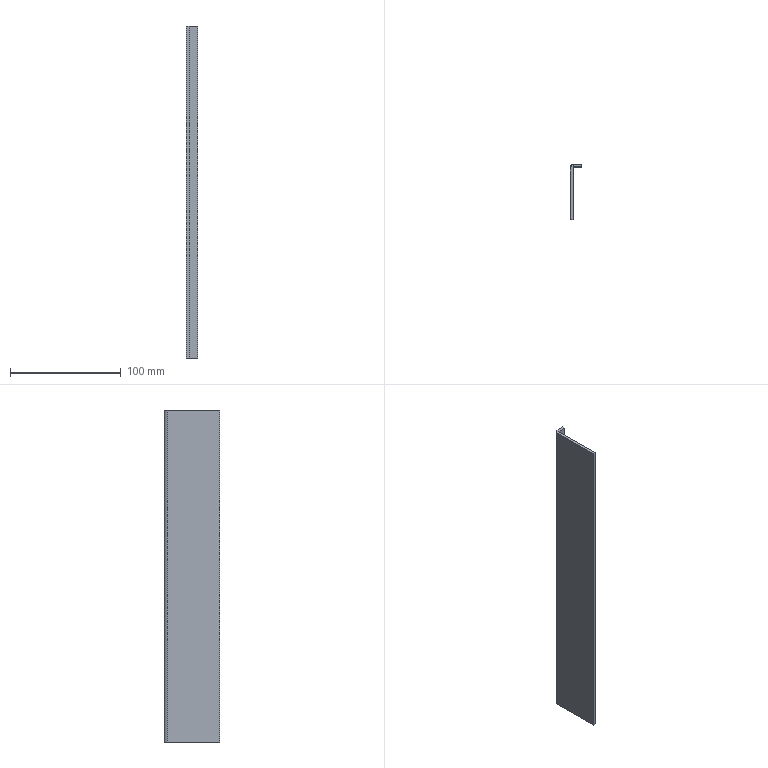Part | SolidWorks | features FlatPattern 1, SMBaseFlange 1, SheetMetal 1 | 1 solid | 14 faces | box 10 x 49.9 x 300 mm | volume 42615 mm3 | plane 12 | cylinder 2 | commonest cylinder face diameters 0.2 x1 5.2 x1
STEP:
#1=CARTESIAN_POINT('',(-7.4,0.,300.));
#2=VERTEX_POINT('',#1);
#3=CARTESIAN_POINT('',(-7.4,-2.5,300.));
#4=VERTEX_POINT('',#3);
#5=CARTESIAN_POINT('',(-7.4,0.,300.));
#6=DIRECTION('',(0.,-1.,0.));
#7=VECTOR('',#6,1000.);
#8=LINE('',#5,#7);
#9=EDGE_CURVE('',#2,#4,#8,.T.);
#10=ORIENTED_EDGE('',*,*,#9,.F.);
#11=CARTESIAN_POINT('',(-10.,-2.6,300.));
#12=VERTEX_POINT('',#11);
#13=CARTESIAN_POINT('',(-7.4,-2.6,300.));
#14=DIRECTION('',(0.,0.,1.));
#15=DIRECTION('',(-1.,0.,0.));
#16=AXIS2_PLACEMENT_3D('',#13,#14,#15);
#17=CIRCLE('',#16,2.6);
#18=EDGE_CURVE('',#2,#12,#17,.T.);
#19=ORIENTED_EDGE('',*,*,#18,.T.);
#20=CARTESIAN_POINT('',(-7.5,-2.6,300.));
#21=VERTEX_POINT('',#20);
#22=CARTESIAN_POINT('',(-7.5,-2.6,300.));
#23=DIRECTION('',(-1.,0.,0.));
#24=VECTOR('',#23,1000.);
#25=LINE('',#22,#24);
#26=EDGE_CURVE('',#21,#12,#25,.T.);
#27=ORIENTED_EDGE('',*,*,#26,.F.);
#28=CARTESIAN_POINT('',(-7.4,-2.6,300.));
#29=DIRECTION('',(0.,0.,1.));
#30=DIRECTION('',(1.,0.,0.));
#31=AXIS2_PLACEMENT_3D('',#28,#29,#30);
#32=CIRCLE('',#31,0.1);
#33=EDGE_CURVE('',#4,#21,#32,.T.);
#34=ORIENTED_EDGE('',*,*,#33,.F.);
#35=EDGE_LOOP('',(#10,#19,#27,#34));
#36=FACE_OUTER_BOUND('',#35,.T.);
#37=CARTESIAN_POINT('',(-7.4,0.,300.));
#38=DIRECTION('',(0.,0.,1.));
#39=DIRECTION('',(1.,0.,0.));
#40=AXIS2_PLACEMENT_3D('',#37,#38,#39);
#41=PLANE('',#40);
#42=ADVANCED_FACE('',(#36),#41,.T.);
#43=CARTESIAN_POINT('',(0.,0.,300.));
#44=VERTEX_POINT('',#43);
#45=CARTESIAN_POINT('',(0.,0.,300.));
#46=DIRECTION('',(-1.,0.,0.));
#47=VECTOR('',#46,1000.);
#48=LINE('',#45,#47);
#49=EDGE_CURVE('',#44,#2,#48,.T.);
#50=ORIENTED_EDGE('',*,*,#49,.T.);
#51=ORIENTED_EDGE('',*,*,#9,.T.);
#52=CARTESIAN_POINT('',(0.,-2.5,300.));
#53=VERTEX_POINT('',#52);
#54=CARTESIAN_POINT('',(0.,-2.5,300.));
#55=DIRECTION('',(-1.,0.,0.));
#56=VECTOR('',#55,1000.);
#57=LINE('',#54,#56);
#58=EDGE_CURVE('',#53,#4,#57,.T.);
#59=ORIENTED_EDGE('',*,*,#58,.F.);
#60=CARTESIAN_POINT('',(0.,0.,300.));
#61=DIRECTION('',(0.,-1.,0.));
#62=VECTOR('',#61,1000.);
#63=LINE('',#60,#62);
#64=EDGE_CURVE('',#44,#53,#63,.T.);
#65=ORIENTED_EDGE('',*,*,#64,.F.);
#66=EDGE_LOOP('',(#50,#51,#59,#65));
#67=FACE_OUTER_BOUND('',#66,.T.);
#68=CARTESIAN_POINT('',(-7.5,-2.6,300.));
#69=DIRECTION('',(0.,0.,1.));
#70=DIRECTION('',(1.,0.,0.));
#71=AXIS2_PLACEMENT_3D('',#68,#69,#70);
#72=PLANE('',#71);
#73=ADVANCED_FACE('',(#67),#72,.T.);
#74=CARTESIAN_POINT('',(-10.,-2.6,0.));
#75=VERTEX_POINT('',#74);
#76=CARTESIAN_POINT('',(-7.5,-2.6,0.));
#77=VERTEX_POINT('',#76);
#78=CARTESIAN_POINT('',(-10.,-2.6,0.));
#79=DIRECTION('',(1.,0.,0.));
#80=VECTOR('',#79,1000.);
#81=LINE('',#78,#80);
#82=EDGE_CURVE('',#75,#77,#81,.T.);
#83=ORIENTED_EDGE('',*,*,#82,.F.);
#84=CARTESIAN_POINT('',(-7.4,0.,0.));
#85=VERTEX_POINT('',#84);
#86=CARTESIAN_POINT('',(-7.4,-2.6,0.));
#87=DIRECTION('',(0.,0.,1.));
#88=DIRECTION('',(-1.,0.,0.));
#89=AXIS2_PLACEMENT_3D('',#86,#87,#88);
#90=CIRCLE('',#89,2.6);
#91=EDGE_CURVE('',#85,#75,#90,.T.);
#92=ORIENTED_EDGE('',*,*,#91,.F.);
#93=CARTESIAN_POINT('',(-7.4,-2.5,0.));
#94=VERTEX_POINT('',#93);
#95=CARTESIAN_POINT('',(-7.4,-2.5,0.));
#96=DIRECTION('',(0.,1.,0.));
#97=VECTOR('',#96,1000.);
#98=LINE('',#95,#97);
#99=EDGE_CURVE('',#94,#85,#98,.T.);
#100=ORIENTED_EDGE('',*,*,#99,.F.);
#101=CARTESIAN_POINT('',(-7.4,-2.6,0.));
#102=DIRECTION('',(0.,0.,1.));
#103=DIRECTION('',(1.,0.,0.));
#104=AXIS2_PLACEMENT_3D('',#101,#102,#103);
#105=CIRCLE('',#104,0.1);
#106=EDGE_CURVE('',#94,#77,#105,.T.);
#107=ORIENTED_EDGE('',*,*,#106,.T.);
#108=EDGE_LOOP('',(#83,#92,#100,#107));
#109=FACE_OUTER_BOUND('',#108,.T.);
#110=CARTESIAN_POINT('',(-10.,-2.6,0.));
#111=DIRECTION('',(0.,0.,-1.));
#112=DIRECTION('',(-1.,0.,0.));
#113=AXIS2_PLACEMENT_3D('',#110,#111,#112);
#114=PLANE('',#113);
#115=ADVANCED_FACE('',(#109),#114,.T.);
#116=CARTESIAN_POINT('',(-10.,-49.9,0.));
#117=VERTEX_POINT('',#116);
#118=CARTESIAN_POINT('',(-10.,0.,0.));
#119=DIRECTION('',(0.,-1.,0.));
#120=VECTOR('',#119,1000.);
#121=LINE('',#118,#120);
#122=EDGE_CURVE('',#75,#117,#121,.T.);
#123=ORIENTED_EDGE('',*,*,#122,.F.);
#124=ORIENTED_EDGE('',*,*,#82,.T.);
#125=CARTESIAN_POINT('',(-7.5,-49.9,0.));
#126=VERTEX_POINT('',#125);
#127=CARTESIAN_POINT('',(-7.5,0.,0.));
#128=DIRECTION('',(0.,-1.,0.));
#129=VECTOR('',#128,1000.);
#130=LINE('',#127,#129);
#131=EDGE_CURVE('',#77,#126,#130,.T.);
#132=ORIENTED_EDGE('',*,*,#131,.T.);
#133=CARTESIAN_POINT('',(-7.5,-49.9,0.));
#134=DIRECTION('',(-1.,0.,0.));
#135=VECTOR('',#134,1000.);
#136=LINE('',#133,#135);
#137=EDGE_CURVE('',#126,#117,#136,.T.);
#138=ORIENTED_EDGE('',*,*,#137,.T.);
#139=EDGE_LOOP('',(#123,#124,#132,#138));
#140=FACE_OUTER_BOUND('',#139,.T.);
#141=CARTESIAN_POINT('',(-7.4,-2.5,0.));
#142=DIRECTION('',(0.,0.,-1.));
#143=DIRECTION('',(-1.,0.,0.));
#144=AXIS2_PLACEMENT_3D('',#141,#142,#143);
#145=PLANE('',#144);
#146=ADVANCED_FACE('',(#140),#145,.T.);
#147=ORIENTED_EDGE('',*,*,#122,.T.);
#148=CARTESIAN_POINT('',(-10.,-49.9,300.));
#149=VERTEX_POINT('',#148);
#150=CARTESIAN_POINT('',(-10.,-49.9,300.));
#151=DIRECTION('',(0.,0.,-1.));
#152=VECTOR('',#151,1000.);
#153=LINE('',#150,#152);
#154=EDGE_CURVE('',#149,#117,#153,.T.);
#155=ORIENTED_EDGE('',*,*,#154,.F.);
#156=CARTESIAN_POINT('',(-10.,0.,300.));
#157=DIRECTION('',(0.,-1.,0.));
#158=VECTOR('',#157,1000.);
#159=LINE('',#156,#158);
#160=EDGE_CURVE('',#12,#149,#159,.T.);
#161=ORIENTED_EDGE('',*,*,#160,.F.);
#162=CARTESIAN_POINT('',(-10.,-2.6,300.));
#163=DIRECTION('',(0.,0.,-1.));
#164=VECTOR('',#163,1000.);
#165=LINE('',#162,#164);
#166=EDGE_CURVE('',#12,#75,#165,.T.);
#167=ORIENTED_EDGE('',*,*,#166,.T.);
#168=EDGE_LOOP('',(#147,#155,#161,#167));
#169=FACE_OUTER_BOUND('',#168,.T.);
#170=CARTESIAN_POINT('',(-10.,0.,300.));
#171=DIRECTION('',(1.,0.,0.));
#172=DIRECTION('',(0.,1.,0.));
#173=AXIS2_PLACEMENT_3D('',#170,#171,#172);
#174=PLANE('',#173);
#175=ADVANCED_FACE('',(#169),#174,.F.);
#176=ORIENTED_EDGE('',*,*,#137,.F.);
#177=CARTESIAN_POINT('',(-7.5,-49.9,300.));
#178=VERTEX_POINT('',#177);
#179=CARTESIAN_POINT('',(-7.5,-49.9,300.));
#180=DIRECTION('',(0.,0.,-1.));
#181=VECTOR('',#180,1000.);
#182=LINE('',#179,#181);
#183=EDGE_CURVE('',#178,#126,#182,.T.);
#184=ORIENTED_EDGE('',*,*,#183,.F.);
#185=CARTESIAN_POINT('',(-7.5,-49.9,300.));
#186=DIRECTION('',(-1.,0.,0.));
#187=VECTOR('',#186,1000.);
#188=LINE('',#185,#187);
#189=EDGE_CURVE('',#178,#149,#188,.T.);
#190=ORIENTED_EDGE('',*,*,#189,.T.);
#191=ORIENTED_EDGE('',*,*,#154,.T.);
#192=EDGE_LOOP('',(#176,#184,#190,#191));
#193=FACE_OUTER_BOUND('',#192,.T.);
#194=CARTESIAN_POINT('',(-7.5,-49.9,300.));
#195=DIRECTION('',(0.,-1.,0.));
#196=DIRECTION('',(0.,0.,-1.));
#197=AXIS2_PLACEMENT_3D('',#194,#195,#196);
#198=PLANE('',#197);
#199=ADVANCED_FACE('',(#193),#198,.T.);
#200=ORIENTED_EDGE('',*,*,#131,.F.);
#201=CARTESIAN_POINT('',(-7.5,-2.6,300.));
#202=DIRECTION('',(0.,0.,-1.));
#203=VECTOR('',#202,1000.);
#204=LINE('',#201,#203);
#205=EDGE_CURVE('',#21,#77,#204,.T.);
#206=ORIENTED_EDGE('',*,*,#205,.F.);
#207=CARTESIAN_POINT('',(-7.5,0.,300.));
#208=DIRECTION('',(0.,-1.,0.));
#209=VECTOR('',#208,1000.);
#210=LINE('',#207,#209);
#211=EDGE_CURVE('',#21,#178,#210,.T.);
#212=ORIENTED_EDGE('',*,*,#211,.T.);
#213=ORIENTED_EDGE('',*,*,#183,.T.);
#214=EDGE_LOOP('',(#200,#206,#212,#213));
#215=FACE_OUTER_BOUND('',#214,.T.);
#216=CARTESIAN_POINT('',(-7.5,0.,300.));
#217=DIRECTION('',(1.,0.,0.));
#218=DIRECTION('',(0.,1.,0.));
#219=AXIS2_PLACEMENT_3D('',#216,#217,#218);
#220=PLANE('',#219);
#221=ADVANCED_FACE('',(#215),#220,.T.);
#222=ORIENTED_EDGE('',*,*,#106,.F.);
#223=CARTESIAN_POINT('',(-7.4,-2.5,300.));
#224=DIRECTION('',(0.,0.,-1.));
#225=VECTOR('',#224,1000.);
#226=LINE('',#223,#225);
#227=EDGE_CURVE('',#4,#94,#226,.T.);
#228=ORIENTED_EDGE('',*,*,#227,.F.);
#229=ORIENTED_EDGE('',*,*,#33,.T.);
#230=ORIENTED_EDGE('',*,*,#205,.T.);
#231=EDGE_LOOP('',(#222,#228,#229,#230));
#232=FACE_OUTER_BOUND('',#231,.T.);
#233=CARTESIAN_POINT('',(-7.4,-2.6,300.));
#234=DIRECTION('',(0.,0.,-1.));
#235=DIRECTION('',(-1.,0.,0.));
#236=AXIS2_PLACEMENT_3D('',#233,#234,#235);
#237=CYLINDRICAL_SURFACE('',#236,0.1);
#238=ADVANCED_FACE('',(#232),#237,.F.);
#239=CARTESIAN_POINT('',(0.,-2.5,0.));
#240=VERTEX_POINT('',#239);
#241=CARTESIAN_POINT('',(0.,-2.5,0.));
#242=DIRECTION('',(-1.,0.,0.));
#243=VECTOR('',#242,1000.);
#244=LINE('',#241,#243);
#245=EDGE_CURVE('',#240,#94,#244,.T.);
#246=ORIENTED_EDGE('',*,*,#245,.F.);
#247=CARTESIAN_POINT('',(0.,-2.5,300.));
#248=DIRECTION('',(0.,0.,-1.));
#249=VECTOR('',#248,1000.);
#250=LINE('',#247,#249);
#251=EDGE_CURVE('',#53,#240,#250,.T.);
#252=ORIENTED_EDGE('',*,*,#251,.F.);
#253=ORIENTED_EDGE('',*,*,#58,.T.);
#254=ORIENTED_EDGE('',*,*,#227,.T.);
#255=EDGE_LOOP('',(#246,#252,#253,#254));
#256=FACE_OUTER_BOUND('',#255,.T.);
#257=CARTESIAN_POINT('',(0.,-2.5,300.));
#258=DIRECTION('',(0.,-1.,0.));
#259=DIRECTION('',(1.,0.,0.));
#260=AXIS2_PLACEMENT_3D('',#257,#258,#259);
#261=PLANE('',#260);
#262=ADVANCED_FACE('',(#256),#261,.T.);
#263=CARTESIAN_POINT('',(0.,0.,0.));
#264=VERTEX_POINT('',#263);
#265=CARTESIAN_POINT('',(0.,0.,0.));
#266=DIRECTION('',(0.,-1.,0.));
#267=VECTOR('',#266,1000.);
#268=LINE('',#265,#267);
#269=EDGE_CURVE('',#264,#240,#268,.T.);
#270=ORIENTED_EDGE('',*,*,#269,.F.);
#271=CARTESIAN_POINT('',(0.,0.,300.));
#272=DIRECTION('',(0.,0.,-1.));
#273=VECTOR('',#272,1000.);
#274=LINE('',#271,#273);
#275=EDGE_CURVE('',#44,#264,#274,.T.);
#276=ORIENTED_EDGE('',*,*,#275,.F.);
#277=ORIENTED_EDGE('',*,*,#64,.T.);
#278=ORIENTED_EDGE('',*,*,#251,.T.);
#279=EDGE_LOOP('',(#270,#276,#277,#278));
#280=FACE_OUTER_BOUND('',#279,.T.);
#281=CARTESIAN_POINT('',(0.,0.,300.));
#282=DIRECTION('',(1.,0.,0.));
#283=DIRECTION('',(0.,1.,0.));
#284=AXIS2_PLACEMENT_3D('',#281,#282,#283);
#285=PLANE('',#284);
#286=ADVANCED_FACE('',(#280),#285,.T.);
#287=CARTESIAN_POINT('',(0.,0.,0.));
#288=DIRECTION('',(-1.,0.,0.));
#289=VECTOR('',#288,1000.);
#290=LINE('',#287,#289);
#291=EDGE_CURVE('',#264,#85,#290,.T.);
#292=ORIENTED_EDGE('',*,*,#291,.T.);
#293=CARTESIAN_POINT('',(-7.4,0.,300.));
#294=DIRECTION('',(0.,0.,-1.));
#295=VECTOR('',#294,1000.);
#296=LINE('',#293,#295);
#297=EDGE_CURVE('',#2,#85,#296,.T.);
#298=ORIENTED_EDGE('',*,*,#297,.F.);
#299=ORIENTED_EDGE('',*,*,#49,.F.);
#300=ORIENTED_EDGE('',*,*,#275,.T.);
#301=EDGE_LOOP('',(#292,#298,#299,#300));
#302=FACE_OUTER_BOUND('',#301,.T.);
#303=CARTESIAN_POINT('',(0.,0.,300.));
#304=DIRECTION('',(0.,-1.,0.));
#305=DIRECTION('',(1.,0.,0.));
#306=AXIS2_PLACEMENT_3D('',#303,#304,#305);
#307=PLANE('',#306);
#308=ADVANCED_FACE('',(#302),#307,.F.);
#309=ORIENTED_EDGE('',*,*,#91,.T.);
#310=ORIENTED_EDGE('',*,*,#166,.F.);
#311=ORIENTED_EDGE('',*,*,#18,.F.);
#312=ORIENTED_EDGE('',*,*,#297,.T.);
#313=EDGE_LOOP('',(#309,#310,#311,#312));
#314=FACE_OUTER_BOUND('',#313,.T.);
#315=CARTESIAN_POINT('',(-7.4,-2.6,300.));
#316=DIRECTION('',(0.,0.,-1.));
#317=DIRECTION('',(-1.,0.,0.));
#318=AXIS2_PLACEMENT_3D('',#315,#316,#317);
#319=CYLINDRICAL_SURFACE('',#318,2.6);
#320=ADVANCED_FACE('',(#314),#319,.T.);
#321=ORIENTED_EDGE('',*,*,#160,.T.);
#322=ORIENTED_EDGE('',*,*,#189,.F.);
#323=ORIENTED_EDGE('',*,*,#211,.F.);
#324=ORIENTED_EDGE('',*,*,#26,.T.);
#325=EDGE_LOOP('',(#321,#322,#323,#324));
#326=FACE_OUTER_BOUND('',#325,.T.);
#327=CARTESIAN_POINT('',(-7.4,-2.6,300.));
#328=DIRECTION('',(0.,0.,1.));
#329=DIRECTION('',(1.,0.,0.));
#330=AXIS2_PLACEMENT_3D('',#327,#328,#329);
#331=PLANE('',#330);
#332=ADVANCED_FACE('',(#326),#331,.T.);
#333=ORIENTED_EDGE('',*,*,#245,.T.);
#334=ORIENTED_EDGE('',*,*,#99,.T.);
#335=ORIENTED_EDGE('',*,*,#291,.F.);
#336=ORIENTED_EDGE('',*,*,#269,.T.);
#337=EDGE_LOOP('',(#333,#334,#335,#336));
#338=FACE_OUTER_BOUND('',#337,.T.);
#339=CARTESIAN_POINT('',(-7.4,-2.6,0.));
#340=DIRECTION('',(0.,0.,1.));
#341=DIRECTION('',(1.,0.,0.));
#342=AXIS2_PLACEMENT_3D('',#339,#340,#341);
#343=PLANE('',#342);
#344=ADVANCED_FACE('',(#338),#343,.F.);
#345=CLOSED_SHELL('',(#42,#73,#115,#146,#175,#199,#221,#238,#262,#286,#308,#320,#332,#344));
#346=MANIFOLD_SOLID_BREP('',#345);
#347=CARTESIAN_POINT('',(0.,0.,0.));
#348=DIRECTION('',(0.,0.,1.));
#349=DIRECTION('',(1.,0.,0.));
#350=AXIS2_PLACEMENT_3D('',#347,#348,#349);
#351=(LENGTH_UNIT()NAMED_UNIT(*)SI_UNIT(.MILLI.,.METRE.));
#352=UNCERTAINTY_MEASURE_WITH_UNIT(LENGTH_MEASURE(0.00001),#351,'','');
#353=(NAMED_UNIT(*)PLANE_ANGLE_UNIT()SI_UNIT($,.RADIAN.));
#354=(NAMED_UNIT(*)SI_UNIT($,.STERADIAN.)SOLID_ANGLE_UNIT());
#355=(GEOMETRIC_REPRESENTATION_CONTEXT(3)GLOBAL_UNCERTAINTY_ASSIGNED_CONTEXT((#352))GLOBAL_UNIT_ASSIGNED_CONTEXT((#351,#353,#354))REPRESENTATION_CONTEXT('',''));
#356=ADVANCED_BREP_SHAPE_REPRESENTATION('',(#346,#350),#355);